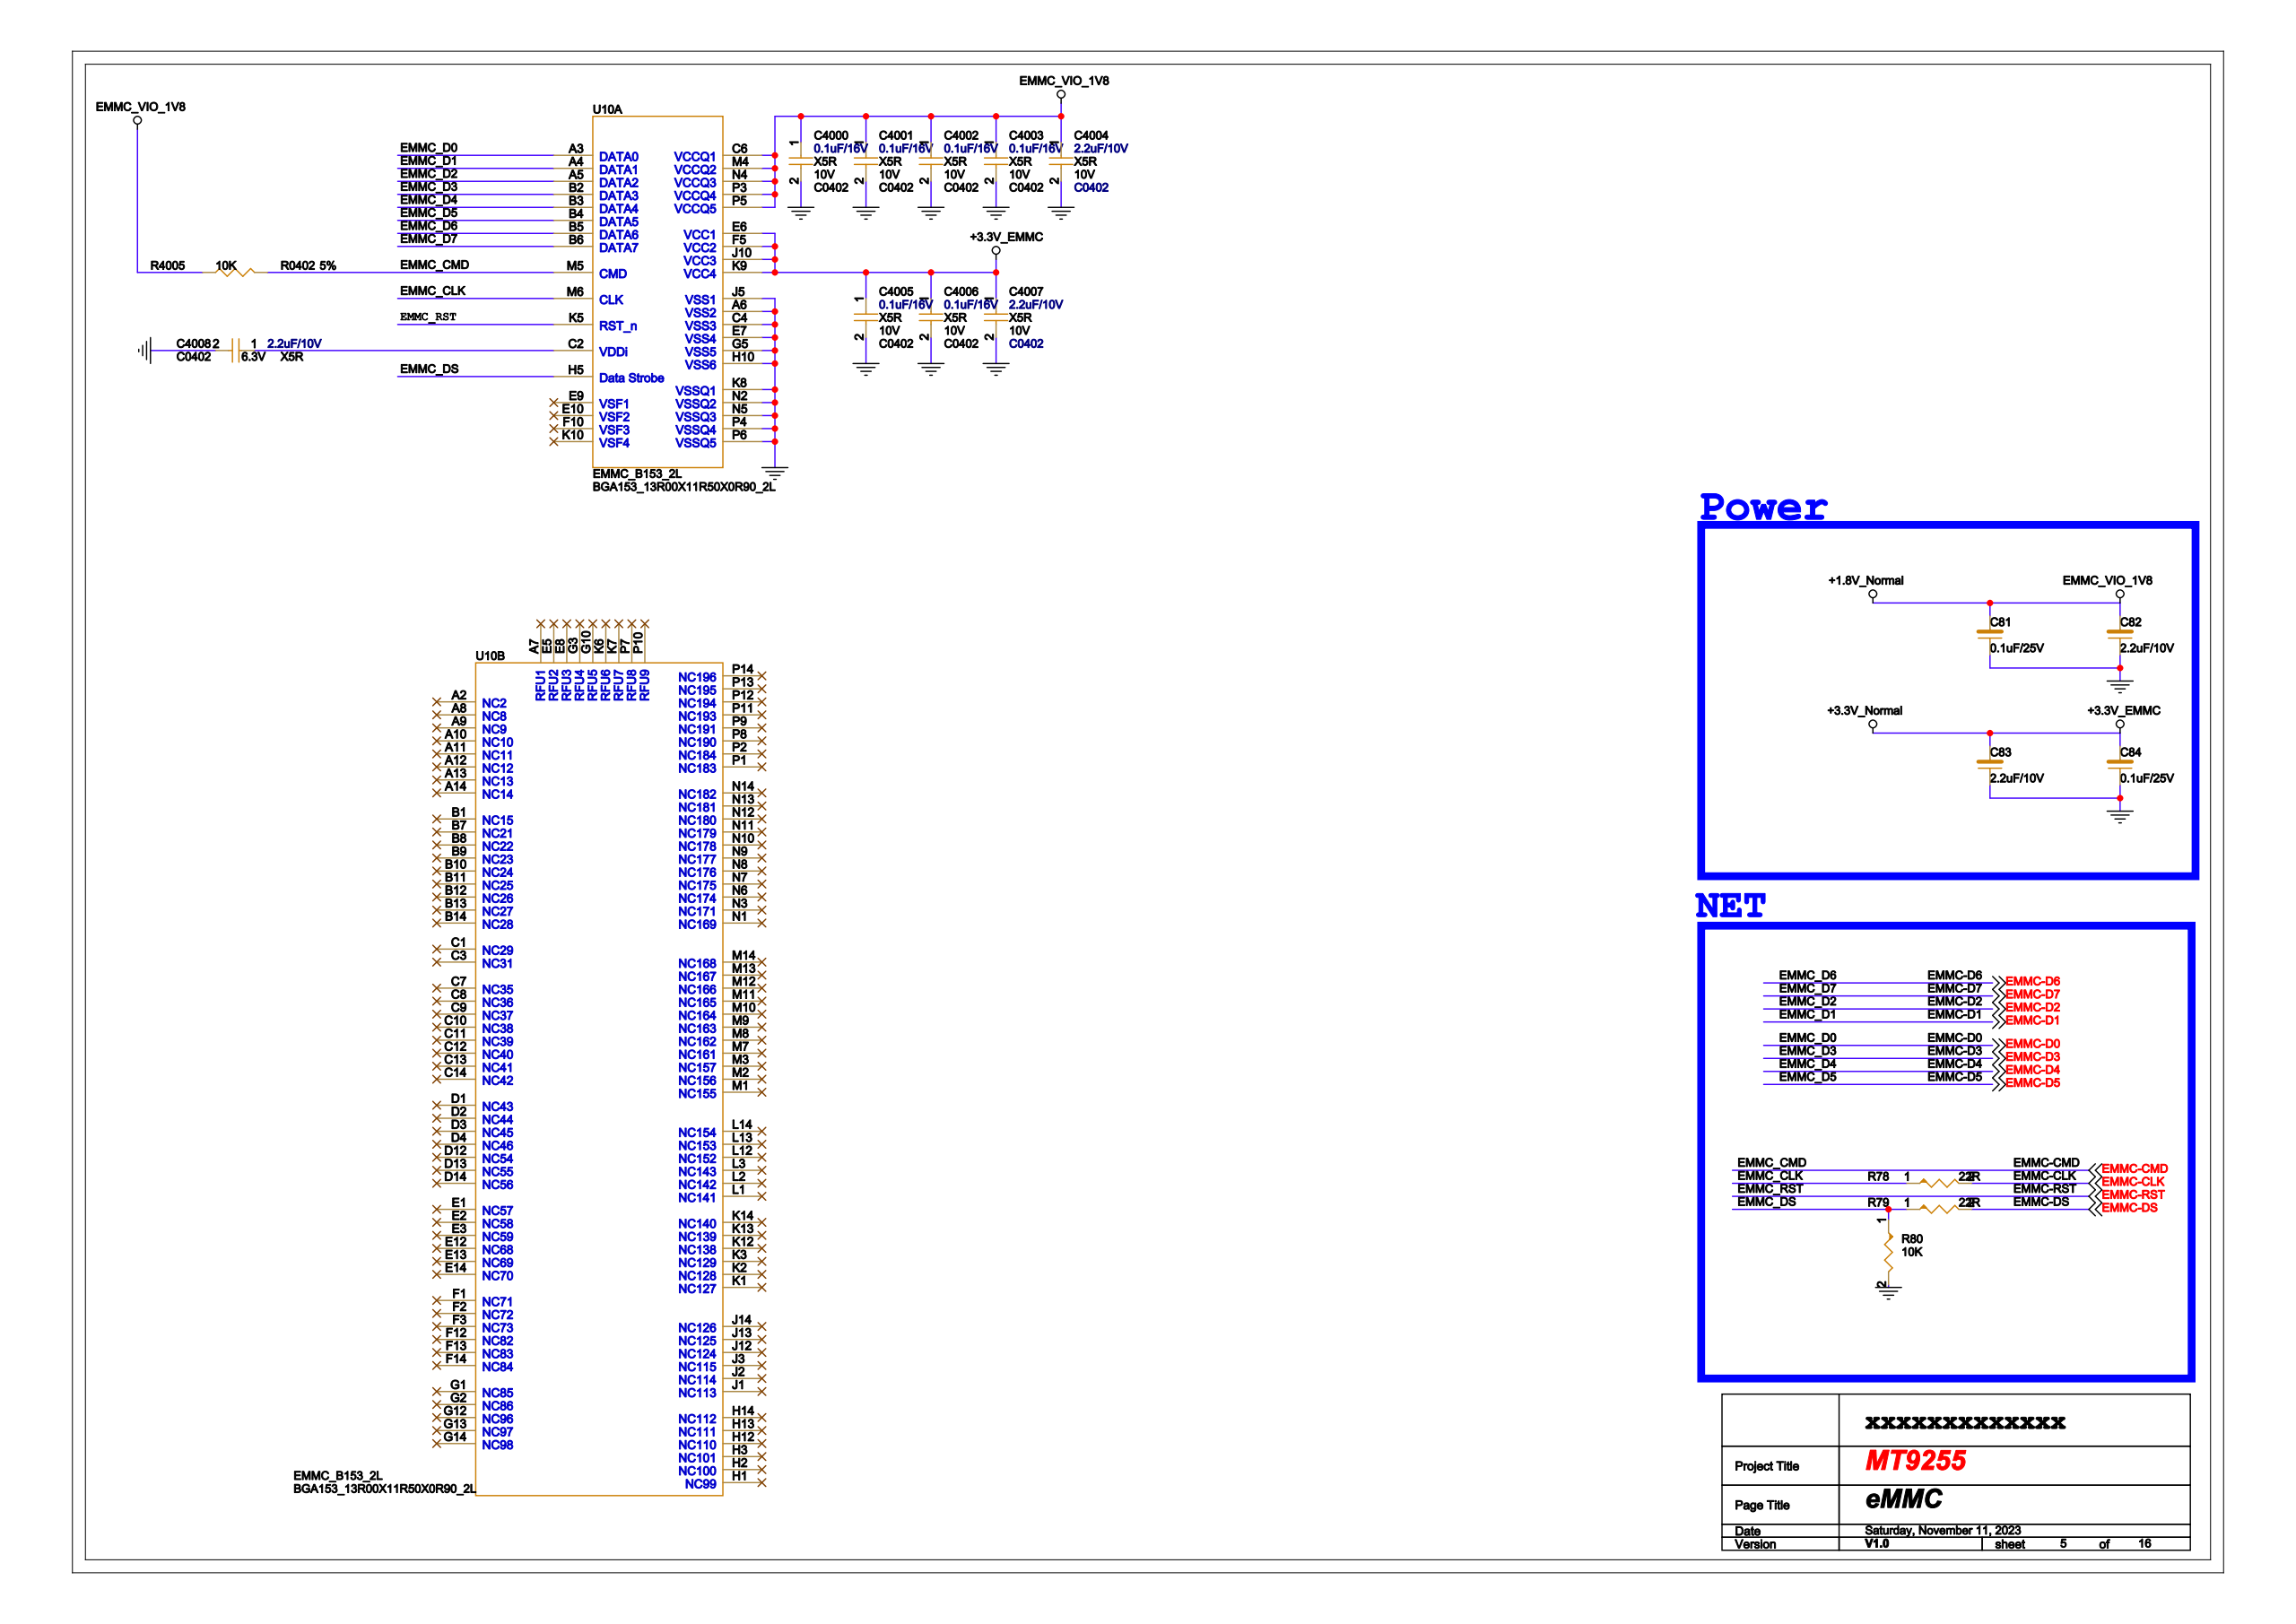Circuit board | Cadence Allegro | 1223 parts | 777 nets | one sheet of the schematic
Parts on this sheet (reference | value | footprint):
C81 | 0.1uF/25V | C0402
C82 | 2.2uF/10V | C0402
C83 | 2.2uF/10V | C0402
C84 | 0.1uF/25V | C0402
C4000 | 0.1uF/16V | C0402
C4001 | 0.1uF/16V | C0402
C4002 | 0.1uF/16V | C0402
C4003 | 0.1uF/16V | C0402
C4004 | 2.2uF/10V | C0402
C4005 | 0.1uF/16V | C0402
C4006 | 0.1uF/16V | C0402
C4007 | 2.2uF/10V | C0402
C4008 | 2.2uF/10V | C0402
P2 | HDMI/90D | HDMI_A
R78 | 22R | R0402
R79 | 22R | R0402
R80 | 10K | R0402
R4005 | 10K | R0402
U10 | EMMC_B153_2L | BGA153_13R00X11R50X0R90_2L
Nets of these parts (net: part-pin ...):
GND: C81-2 C82-2 C83-2 C84-2 C4000-2 C4001-2 C4002-2 C4003-2 C4004-2 C4005-2 C4006-2 C4007-2 C4008-2 R80-2 P2-2 P2-5 P2-11 U10-A6 U10-C4 U10-E7 U10-G5 U10-H10 U10-J5 U10-K8 U10-N2 U10-N5 U10-P4 U10-P6
+3.3V_EMMC: C83-1 C84-1 C4005-1 C4006-1 C4007-1 U10-E6 U10-F5 U10-J10 U10-K9
+1.8V_NORMAL: C81-1 C82-1 C4000-1 C4001-1 C4002-1 C4003-1 C4004-1 R4005-1 U10-C6 U10-M4 U10-N4 U10-P3 U10-P5
N24437802: C4008-1 U10-C2
EMMC-CMD: R4005-2 U10-M5
EMMC_DS: R79-1 R80-1 U10-H5
EMMC_CLK: R78-1 U10-M6
EMMC-CLK: R78-2
EMMC-DS: R79-2
EMMC-D0: U10-A3
EMMC-D1: U10-A4
EMMC-D2: U10-A5
EMMC-D3: U10-B2
EMMC-D4: U10-B3
EMMC-D5: U10-B4
EMMC-D6: U10-B5
EMMC-D7: U10-B6
EMMC-RST: U10-K5